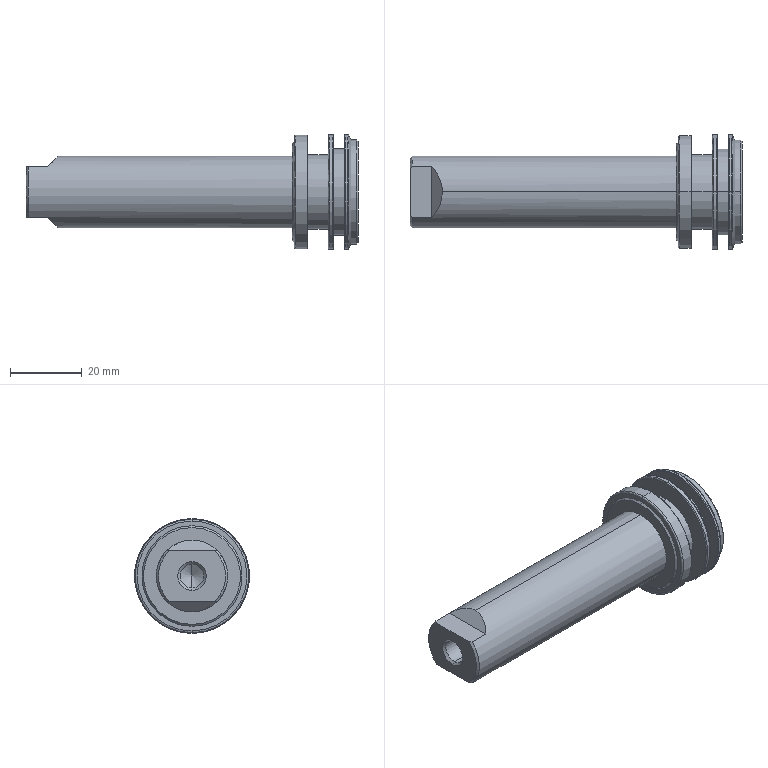Part | SolidWorks | features BaseBody 1 | 1 solid | 52 faces | box 92.5 x 32 x 32 mm | volume 32646 mm3 | cylinder 16 | cone 14 | plane 12 | spline 10 | commonest cylinder face diameters 32 x4 6.647 x2 20 x2 20.82 x2 24 x2 29 x2